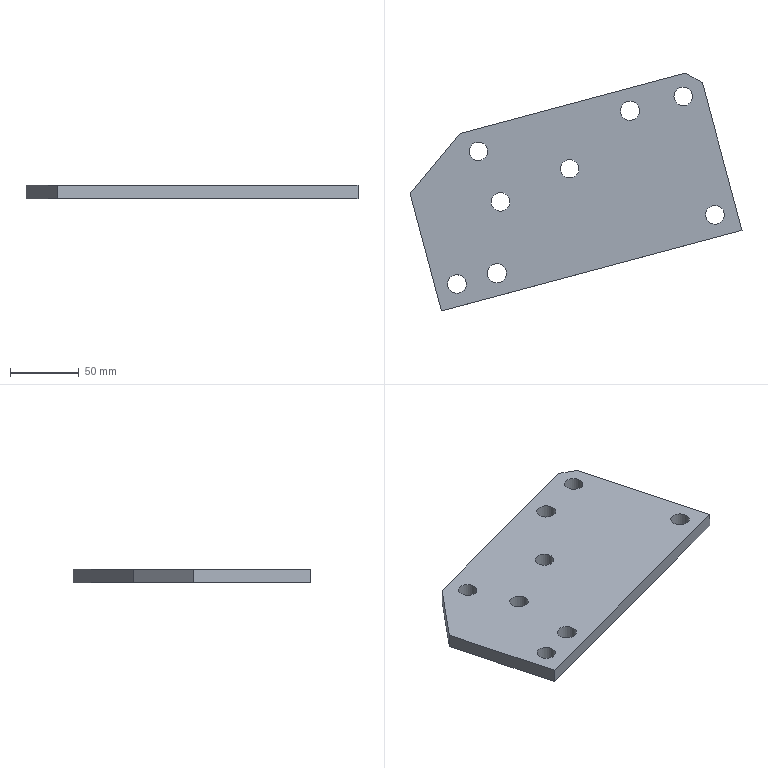Part | NX | features 6 2 | 1 solid | 16 faces | box 241.063 x 172.782 x 10 mm | volume 253614 mm3 | plane 8 | cylinder 8 | commonest cylinder face diameters 13.5 x6 14.001 x2
STEP:
#1=CARTESIAN_POINT('',(606.241,-48.522,101.));
#2=VERTEX_POINT('',#1);
#3=CARTESIAN_POINT('',(599.491,-48.522,101.));
#4=DIRECTION('',(0.,0.,1.));
#5=DIRECTION('',(1.,0.,0.));
#6=AXIS2_PLACEMENT_3D('',#3,#4,#5);
#7=CIRCLE('',#6,6.75);
#8=EDGE_CURVE('',#2,#2,#7,.T.);
#9=ORIENTED_EDGE('',*,*,#8,.F.);
#10=EDGE_LOOP('',(#9));
#11=FACE_BOUND('',#10,.T.);
#12=CARTESIAN_POINT('',(570.07,1.105,101.));
#13=VERTEX_POINT('',#12);
#14=CARTESIAN_POINT('',(533.734,-42.843,101.));
#15=VERTEX_POINT('',#14);
#16=CARTESIAN_POINT('',(534.187,-42.295,101.));
#17=DIRECTION('',(-0.6372,-0.7707,0.));
#18=VECTOR('',#17,1000.);
#19=LINE('',#16,#18);
#20=EDGE_CURVE('',#13,#15,#19,.T.);
#21=ORIENTED_EDGE('',*,*,#20,.T.);
#22=CARTESIAN_POINT('',(556.498,-127.8,101.));
#23=VERTEX_POINT('',#22);
#24=CARTESIAN_POINT('',(542.781,-76.606,101.));
#25=DIRECTION('',(-0.2588,0.9659,0.));
#26=VECTOR('',#25,1000.);
#27=LINE('',#24,#26);
#28=EDGE_CURVE('',#23,#15,#27,.T.);
#29=ORIENTED_EDGE('',*,*,#28,.F.);
#30=CARTESIAN_POINT('',(774.797,-69.307,101.));
#31=VERTEX_POINT('',#30);
#32=CARTESIAN_POINT('',(665.648,-98.554,101.));
#33=DIRECTION('',(-0.9659,-0.2588,0.));
#34=VECTOR('',#33,1000.);
#35=LINE('',#32,#34);
#36=EDGE_CURVE('',#31,#23,#35,.T.);
#37=ORIENTED_EDGE('',*,*,#36,.F.);
#38=CARTESIAN_POINT('',(746.068,37.911,101.));
#39=VERTEX_POINT('',#38);
#40=CARTESIAN_POINT('',(761.08,-18.113,101.));
#41=DIRECTION('',(0.2588,-0.9659,0.));
#42=VECTOR('',#41,1000.);
#43=LINE('',#40,#42);
#44=EDGE_CURVE('',#39,#31,#43,.T.);
#45=ORIENTED_EDGE('',*,*,#44,.F.);
#46=CARTESIAN_POINT('',(733.821,44.982,101.));
#47=VERTEX_POINT('',#46);
#48=CARTESIAN_POINT('',(304.806,292.674,101.));
#49=DIRECTION('',(-0.866,0.5,0.));
#50=VECTOR('',#49,1000.);
#51=LINE('',#48,#50);
#52=EDGE_CURVE('',#39,#47,#51,.T.);
#53=ORIENTED_EDGE('',*,*,#52,.T.);
#54=CARTESIAN_POINT('',(634.331,18.323,101.));
#55=DIRECTION('',(0.9659,0.2588,0.));
#56=VECTOR('',#55,1000.);
#57=LINE('',#54,#56);
#58=EDGE_CURVE('',#13,#47,#57,.T.);
#59=ORIENTED_EDGE('',*,*,#58,.F.);
#60=EDGE_LOOP('',(#21,#29,#37,#45,#53,#59));
#61=FACE_BOUND('',#60,.T.);
#62=CARTESIAN_POINT('',(603.552,-98.628,101.));
#63=VERTEX_POINT('',#62);
#64=CARTESIAN_POINT('',(596.79,-100.44,101.));
#65=DIRECTION('',(0.,0.,-1.));
#66=DIRECTION('',(0.9659,0.2588,0.));
#67=AXIS2_PLACEMENT_3D('',#64,#65,#66);
#68=CIRCLE('',#67,7.);
#69=EDGE_CURVE('',#63,#63,#68,.T.);
#70=ORIENTED_EDGE('',*,*,#69,.T.);
#71=EDGE_LOOP('',(#70));
#72=FACE_BOUND('',#71,.T.);
#73=CARTESIAN_POINT('',(761.721,-56.246,101.));
#74=VERTEX_POINT('',#73);
#75=CARTESIAN_POINT('',(755.201,-57.993,101.));
#76=DIRECTION('',(0.,0.,-1.));
#77=DIRECTION('',(0.9659,0.2588,0.));
#78=AXIS2_PLACEMENT_3D('',#75,#76,#77);
#79=CIRCLE('',#78,6.75);
#80=EDGE_CURVE('',#74,#74,#79,.T.);
#81=ORIENTED_EDGE('',*,*,#80,.T.);
#82=EDGE_LOOP('',(#81));
#83=FACE_BOUND('',#82,.T.);
#84=CARTESIAN_POINT('',(574.332,-106.457,101.));
#85=VERTEX_POINT('',#84);
#86=CARTESIAN_POINT('',(567.812,-108.204,101.));
#87=DIRECTION('',(0.,0.,-1.));
#88=DIRECTION('',(0.9659,0.2588,0.));
#89=AXIS2_PLACEMENT_3D('',#86,#87,#88);
#90=CIRCLE('',#89,6.75);
#91=EDGE_CURVE('',#85,#85,#90,.T.);
#92=ORIENTED_EDGE('',*,*,#91,.T.);
#93=EDGE_LOOP('',(#92));
#94=FACE_BOUND('',#93,.T.);
#95=CARTESIAN_POINT('',(738.687,29.721,101.));
#96=VERTEX_POINT('',#95);
#97=CARTESIAN_POINT('',(732.167,27.974,101.));
#98=DIRECTION('',(0.,0.,-1.));
#99=DIRECTION('',(0.9659,0.2588,0.));
#100=AXIS2_PLACEMENT_3D('',#97,#98,#99);
#101=CIRCLE('',#100,6.75);
#102=EDGE_CURVE('',#96,#96,#101,.T.);
#103=ORIENTED_EDGE('',*,*,#102,.T.);
#104=EDGE_LOOP('',(#103));
#105=FACE_BOUND('',#104,.T.);
#106=CARTESIAN_POINT('',(589.934,-10.137,101.));
#107=VERTEX_POINT('',#106);
#108=CARTESIAN_POINT('',(583.414,-11.884,101.));
#109=DIRECTION('',(0.,0.,-1.));
#110=DIRECTION('',(0.9659,0.2588,0.));
#111=AXIS2_PLACEMENT_3D('',#108,#109,#110);
#112=CIRCLE('',#111,6.75);
#113=EDGE_CURVE('',#107,#107,#112,.T.);
#114=ORIENTED_EDGE('',*,*,#113,.T.);
#115=EDGE_LOOP('',(#114));
#116=FACE_BOUND('',#115,.T.);
#117=CARTESIAN_POINT('',(700.292,19.433,101.));
#118=VERTEX_POINT('',#117);
#119=CARTESIAN_POINT('',(693.53,17.621,101.));
#120=DIRECTION('',(0.,0.,-1.));
#121=DIRECTION('',(0.9659,0.2588,0.));
#122=AXIS2_PLACEMENT_3D('',#119,#120,#121);
#123=CIRCLE('',#122,7.);
#124=EDGE_CURVE('',#118,#118,#123,.T.);
#125=ORIENTED_EDGE('',*,*,#124,.T.);
#126=EDGE_LOOP('',(#125));
#127=FACE_BOUND('',#126,.T.);
#128=CARTESIAN_POINT('',(656.441,-24.522,101.));
#129=VERTEX_POINT('',#128);
#130=CARTESIAN_POINT('',(649.691,-24.522,101.));
#131=DIRECTION('',(0.,0.,1.));
#132=DIRECTION('',(1.,0.,0.));
#133=AXIS2_PLACEMENT_3D('',#130,#131,#132);
#134=CIRCLE('',#133,6.75);
#135=EDGE_CURVE('',#129,#129,#134,.T.);
#136=ORIENTED_EDGE('',*,*,#135,.F.);
#137=EDGE_LOOP('',(#136));
#138=FACE_BOUND('',#137,.T.);
#139=CARTESIAN_POINT('',(189.696,93.298,101.));
#140=DIRECTION('',(0.,0.,1.));
#141=DIRECTION('',(-0.9848,0.1736,0.));
#142=AXIS2_PLACEMENT_3D('',#139,#140,#141);
#143=PLANE('',#142);
#144=ADVANCED_FACE('',(#11,#61,#72,#83,#94,#105,#116,#127,#138),#143,.T.);
#145=CARTESIAN_POINT('',(592.741,-48.522,91.));
#146=VERTEX_POINT('',#145);
#147=CARTESIAN_POINT('',(599.491,-48.522,91.));
#148=DIRECTION('',(0.,0.,1.));
#149=DIRECTION('',(-1.,0.,0.));
#150=AXIS2_PLACEMENT_3D('',#147,#148,#149);
#151=CIRCLE('',#150,6.75);
#152=EDGE_CURVE('',#146,#146,#151,.T.);
#153=ORIENTED_EDGE('',*,*,#152,.T.);
#154=EDGE_LOOP('',(#153));
#155=FACE_BOUND('',#154,.T.);
#156=CARTESIAN_POINT('',(570.07,1.105,91.));
#157=VERTEX_POINT('',#156);
#158=CARTESIAN_POINT('',(533.734,-42.843,91.));
#159=VERTEX_POINT('',#158);
#160=CARTESIAN_POINT('',(579.507,12.519,91.));
#161=DIRECTION('',(-0.6372,-0.7707,0.));
#162=VECTOR('',#161,1000.);
#163=LINE('',#160,#162);
#164=EDGE_CURVE('',#157,#159,#163,.T.);
#165=ORIENTED_EDGE('',*,*,#164,.F.);
#166=CARTESIAN_POINT('',(733.821,44.982,91.));
#167=VERTEX_POINT('',#166);
#168=CARTESIAN_POINT('',(634.331,18.323,91.));
#169=DIRECTION('',(-0.9659,-0.2588,0.));
#170=VECTOR('',#169,1000.);
#171=LINE('',#168,#170);
#172=EDGE_CURVE('',#167,#157,#171,.T.);
#173=ORIENTED_EDGE('',*,*,#172,.F.);
#174=CARTESIAN_POINT('',(746.068,37.911,91.));
#175=VERTEX_POINT('',#174);
#176=CARTESIAN_POINT('',(712.388,57.356,91.));
#177=DIRECTION('',(0.866,-0.5,0.));
#178=VECTOR('',#177,1000.);
#179=LINE('',#176,#178);
#180=EDGE_CURVE('',#167,#175,#179,.T.);
#181=ORIENTED_EDGE('',*,*,#180,.T.);
#182=CARTESIAN_POINT('',(774.797,-69.307,91.));
#183=VERTEX_POINT('',#182);
#184=CARTESIAN_POINT('',(761.08,-18.113,91.));
#185=DIRECTION('',(-0.2588,0.9659,0.));
#186=VECTOR('',#185,1000.);
#187=LINE('',#184,#186);
#188=EDGE_CURVE('',#183,#175,#187,.T.);
#189=ORIENTED_EDGE('',*,*,#188,.F.);
#190=CARTESIAN_POINT('',(556.498,-127.8,91.));
#191=VERTEX_POINT('',#190);
#192=CARTESIAN_POINT('',(665.648,-98.554,91.));
#193=DIRECTION('',(0.9659,0.2588,0.));
#194=VECTOR('',#193,1000.);
#195=LINE('',#192,#194);
#196=EDGE_CURVE('',#191,#183,#195,.T.);
#197=ORIENTED_EDGE('',*,*,#196,.F.);
#198=CARTESIAN_POINT('',(542.781,-76.606,91.));
#199=DIRECTION('',(0.2588,-0.9659,0.));
#200=VECTOR('',#199,1000.);
#201=LINE('',#198,#200);
#202=EDGE_CURVE('',#159,#191,#201,.T.);
#203=ORIENTED_EDGE('',*,*,#202,.F.);
#204=EDGE_LOOP('',(#165,#173,#181,#189,#197,#203));
#205=FACE_BOUND('',#204,.T.);
#206=CARTESIAN_POINT('',(603.552,-98.628,91.));
#207=VERTEX_POINT('',#206);
#208=CARTESIAN_POINT('',(596.79,-100.44,91.));
#209=DIRECTION('',(0.,0.,1.));
#210=DIRECTION('',(0.9659,0.2588,0.));
#211=AXIS2_PLACEMENT_3D('',#208,#209,#210);
#212=CIRCLE('',#211,7.);
#213=EDGE_CURVE('',#207,#207,#212,.T.);
#214=ORIENTED_EDGE('',*,*,#213,.T.);
#215=EDGE_LOOP('',(#214));
#216=FACE_BOUND('',#215,.T.);
#217=CARTESIAN_POINT('',(761.721,-56.246,91.));
#218=VERTEX_POINT('',#217);
#219=CARTESIAN_POINT('',(755.201,-57.993,91.));
#220=DIRECTION('',(0.,0.,1.));
#221=DIRECTION('',(0.9659,0.2588,0.));
#222=AXIS2_PLACEMENT_3D('',#219,#220,#221);
#223=CIRCLE('',#222,6.75);
#224=EDGE_CURVE('',#218,#218,#223,.T.);
#225=ORIENTED_EDGE('',*,*,#224,.T.);
#226=EDGE_LOOP('',(#225));
#227=FACE_BOUND('',#226,.T.);
#228=CARTESIAN_POINT('',(574.332,-106.457,91.));
#229=VERTEX_POINT('',#228);
#230=CARTESIAN_POINT('',(567.812,-108.204,91.));
#231=DIRECTION('',(0.,0.,1.));
#232=DIRECTION('',(0.9659,0.2588,0.));
#233=AXIS2_PLACEMENT_3D('',#230,#231,#232);
#234=CIRCLE('',#233,6.75);
#235=EDGE_CURVE('',#229,#229,#234,.T.);
#236=ORIENTED_EDGE('',*,*,#235,.T.);
#237=EDGE_LOOP('',(#236));
#238=FACE_BOUND('',#237,.T.);
#239=CARTESIAN_POINT('',(738.687,29.721,91.));
#240=VERTEX_POINT('',#239);
#241=CARTESIAN_POINT('',(732.167,27.974,91.));
#242=DIRECTION('',(0.,0.,1.));
#243=DIRECTION('',(0.9659,0.2588,0.));
#244=AXIS2_PLACEMENT_3D('',#241,#242,#243);
#245=CIRCLE('',#244,6.75);
#246=EDGE_CURVE('',#240,#240,#245,.T.);
#247=ORIENTED_EDGE('',*,*,#246,.T.);
#248=EDGE_LOOP('',(#247));
#249=FACE_BOUND('',#248,.T.);
#250=CARTESIAN_POINT('',(589.934,-10.137,91.));
#251=VERTEX_POINT('',#250);
#252=CARTESIAN_POINT('',(583.414,-11.884,91.));
#253=DIRECTION('',(0.,0.,1.));
#254=DIRECTION('',(0.9659,0.2588,0.));
#255=AXIS2_PLACEMENT_3D('',#252,#253,#254);
#256=CIRCLE('',#255,6.75);
#257=EDGE_CURVE('',#251,#251,#256,.T.);
#258=ORIENTED_EDGE('',*,*,#257,.T.);
#259=EDGE_LOOP('',(#258));
#260=FACE_BOUND('',#259,.T.);
#261=CARTESIAN_POINT('',(700.292,19.433,91.));
#262=VERTEX_POINT('',#261);
#263=CARTESIAN_POINT('',(693.53,17.621,91.));
#264=DIRECTION('',(0.,0.,1.));
#265=DIRECTION('',(0.9659,0.2588,0.));
#266=AXIS2_PLACEMENT_3D('',#263,#264,#265);
#267=CIRCLE('',#266,7.);
#268=EDGE_CURVE('',#262,#262,#267,.T.);
#269=ORIENTED_EDGE('',*,*,#268,.T.);
#270=EDGE_LOOP('',(#269));
#271=FACE_BOUND('',#270,.T.);
#272=CARTESIAN_POINT('',(642.941,-24.522,91.));
#273=VERTEX_POINT('',#272);
#274=CARTESIAN_POINT('',(649.691,-24.522,91.));
#275=DIRECTION('',(0.,0.,1.));
#276=DIRECTION('',(-1.,0.,0.));
#277=AXIS2_PLACEMENT_3D('',#274,#275,#276);
#278=CIRCLE('',#277,6.75);
#279=EDGE_CURVE('',#273,#273,#278,.T.);
#280=ORIENTED_EDGE('',*,*,#279,.T.);
#281=EDGE_LOOP('',(#280));
#282=FACE_BOUND('',#281,.T.);
#283=CARTESIAN_POINT('',(651.93,-47.36,91.));
#284=DIRECTION('',(0.,0.,-1.));
#285=DIRECTION('',(0.9659,0.2588,0.));
#286=AXIS2_PLACEMENT_3D('',#283,#284,#285);
#287=PLANE('',#286);
#288=ADVANCED_FACE('',(#155,#205,#216,#227,#238,#249,#260,#271,#282),#287,.T.);
#289=CARTESIAN_POINT('',(774.797,-69.307,91.));
#290=DIRECTION('',(0.,0.,1.));
#291=VECTOR('',#290,1000.);
#292=LINE('',#289,#291);
#293=EDGE_CURVE('',#183,#31,#292,.T.);
#294=ORIENTED_EDGE('',*,*,#293,.T.);
#295=ORIENTED_EDGE('',*,*,#36,.T.);
#296=CARTESIAN_POINT('',(556.498,-127.8,91.));
#297=DIRECTION('',(0.,0.,1.));
#298=VECTOR('',#297,1000.);
#299=LINE('',#296,#298);
#300=EDGE_CURVE('',#191,#23,#299,.T.);
#301=ORIENTED_EDGE('',*,*,#300,.F.);
#302=ORIENTED_EDGE('',*,*,#196,.T.);
#303=EDGE_LOOP('',(#294,#295,#301,#302));
#304=FACE_BOUND('',#303,.T.);
#305=CARTESIAN_POINT('',(665.648,-98.554,91.));
#306=DIRECTION('',(0.2588,-0.9659,0.));
#307=DIRECTION('',(0.,0.,1.));
#308=AXIS2_PLACEMENT_3D('',#305,#306,#307);
#309=PLANE('',#308);
#310=ADVANCED_FACE('',(#304),#309,.T.);
#311=CARTESIAN_POINT('',(533.734,-42.843,91.));
#312=DIRECTION('',(0.,0.,1.));
#313=VECTOR('',#312,1000.);
#314=LINE('',#311,#313);
#315=EDGE_CURVE('',#159,#15,#314,.T.);
#316=ORIENTED_EDGE('',*,*,#315,.F.);
#317=ORIENTED_EDGE('',*,*,#202,.T.);
#318=ORIENTED_EDGE('',*,*,#300,.T.);
#319=ORIENTED_EDGE('',*,*,#28,.T.);
#320=EDGE_LOOP('',(#316,#317,#318,#319));
#321=FACE_BOUND('',#320,.T.);
#322=CARTESIAN_POINT('',(542.781,-76.606,91.));
#323=DIRECTION('',(-0.9659,-0.2588,0.));
#324=DIRECTION('',(0.,0.,-1.));
#325=AXIS2_PLACEMENT_3D('',#322,#323,#324);
#326=PLANE('',#325);
#327=ADVANCED_FACE('',(#321),#326,.T.);
#328=CARTESIAN_POINT('',(570.07,1.105,91.));
#329=DIRECTION('',(0.,0.,-1.));
#330=VECTOR('',#329,1000.);
#331=LINE('',#328,#330);
#332=EDGE_CURVE('',#13,#157,#331,.T.);
#333=ORIENTED_EDGE('',*,*,#332,.F.);
#334=ORIENTED_EDGE('',*,*,#58,.T.);
#335=CARTESIAN_POINT('',(733.821,44.982,91.));
#336=DIRECTION('',(0.,0.,-1.));
#337=VECTOR('',#336,1000.);
#338=LINE('',#335,#337);
#339=EDGE_CURVE('',#47,#167,#338,.T.);
#340=ORIENTED_EDGE('',*,*,#339,.T.);
#341=ORIENTED_EDGE('',*,*,#172,.T.);
#342=EDGE_LOOP('',(#333,#334,#340,#341));
#343=FACE_BOUND('',#342,.T.);
#344=CARTESIAN_POINT('',(634.331,18.323,91.));
#345=DIRECTION('',(-0.2588,0.9659,0.));
#346=DIRECTION('',(0.,0.,-1.));
#347=AXIS2_PLACEMENT_3D('',#344,#345,#346);
#348=PLANE('',#347);
#349=ADVANCED_FACE('',(#343),#348,.T.);
#350=ORIENTED_EDGE('',*,*,#188,.T.);
#351=CARTESIAN_POINT('',(746.068,37.911,91.));
#352=DIRECTION('',(0.,0.,1.));
#353=VECTOR('',#352,1000.);
#354=LINE('',#351,#353);
#355=EDGE_CURVE('',#175,#39,#354,.T.);
#356=ORIENTED_EDGE('',*,*,#355,.T.);
#357=ORIENTED_EDGE('',*,*,#44,.T.);
#358=ORIENTED_EDGE('',*,*,#293,.F.);
#359=EDGE_LOOP('',(#350,#356,#357,#358));
#360=FACE_BOUND('',#359,.T.);
#361=CARTESIAN_POINT('',(761.08,-18.113,91.));
#362=DIRECTION('',(0.9659,0.2588,0.));
#363=DIRECTION('',(0.,0.,1.));
#364=AXIS2_PLACEMENT_3D('',#361,#362,#363);
#365=PLANE('',#364);
#366=ADVANCED_FACE('',(#360),#365,.T.);
#367=ORIENTED_EDGE('',*,*,#91,.F.);
#368=EDGE_LOOP('',(#367));
#369=FACE_BOUND('',#368,.T.);
#370=ORIENTED_EDGE('',*,*,#235,.F.);
#371=EDGE_LOOP('',(#370));
#372=FACE_BOUND('',#371,.T.);
#373=CARTESIAN_POINT('',(567.812,-108.204,91.));
#374=DIRECTION('',(0.,0.,1.));
#375=DIRECTION('',(-0.9659,-0.2588,0.));
#376=AXIS2_PLACEMENT_3D('',#373,#374,#375);
#377=CYLINDRICAL_SURFACE('',#376,6.75);
#378=ADVANCED_FACE('',(#369,#372),#377,.F.);
#379=ORIENTED_EDGE('',*,*,#102,.F.);
#380=EDGE_LOOP('',(#379));
#381=FACE_BOUND('',#380,.T.);
#382=ORIENTED_EDGE('',*,*,#246,.F.);
#383=EDGE_LOOP('',(#382));
#384=FACE_BOUND('',#383,.T.);
#385=CARTESIAN_POINT('',(732.167,27.974,91.));
#386=DIRECTION('',(0.,0.,1.));
#387=DIRECTION('',(-0.9659,-0.2588,0.));
#388=AXIS2_PLACEMENT_3D('',#385,#386,#387);
#389=CYLINDRICAL_SURFACE('',#388,6.75);
#390=ADVANCED_FACE('',(#381,#384),#389,.F.);
#391=ORIENTED_EDGE('',*,*,#80,.F.);
#392=EDGE_LOOP('',(#391));
#393=FACE_BOUND('',#392,.T.);
#394=ORIENTED_EDGE('',*,*,#224,.F.);
#395=EDGE_LOOP('',(#394));
#396=FACE_BOUND('',#395,.T.);
#397=CARTESIAN_POINT('',(755.201,-57.993,91.));
#398=DIRECTION('',(0.,0.,1.));
#399=DIRECTION('',(-0.9659,-0.2588,0.));
#400=AXIS2_PLACEMENT_3D('',#397,#398,#399);
#401=CYLINDRICAL_SURFACE('',#400,6.75);
#402=ADVANCED_FACE('',(#393,#396),#401,.F.);
#403=ORIENTED_EDGE('',*,*,#113,.F.);
#404=EDGE_LOOP('',(#403));
#405=FACE_BOUND('',#404,.T.);
#406=ORIENTED_EDGE('',*,*,#257,.F.);
#407=EDGE_LOOP('',(#406));
#408=FACE_BOUND('',#407,.T.);
#409=CARTESIAN_POINT('',(583.414,-11.884,91.));
#410=DIRECTION('',(0.,0.,1.));
#411=DIRECTION('',(-0.9659,-0.2588,0.));
#412=AXIS2_PLACEMENT_3D('',#409,#410,#411);
#413=CYLINDRICAL_SURFACE('',#412,6.75);
#414=ADVANCED_FACE('',(#405,#408),#413,.F.);
#415=ORIENTED_EDGE('',*,*,#69,.F.);
#416=EDGE_LOOP('',(#415));
#417=FACE_BOUND('',#416,.T.);
#418=ORIENTED_EDGE('',*,*,#213,.F.);
#419=EDGE_LOOP('',(#418));
#420=FACE_BOUND('',#419,.T.);
#421=CARTESIAN_POINT('',(596.79,-100.44,91.));
#422=DIRECTION('',(0.,0.,1.));
#423=DIRECTION('',(-0.9659,-0.2588,0.));
#424=AXIS2_PLACEMENT_3D('',#421,#422,#423);
#425=CYLINDRICAL_SURFACE('',#424,7.);
#426=ADVANCED_FACE('',(#417,#420),#425,.F.);
#427=ORIENTED_EDGE('',*,*,#124,.F.);
#428=EDGE_LOOP('',(#427));
#429=FACE_BOUND('',#428,.T.);
#430=ORIENTED_EDGE('',*,*,#268,.F.);
#431=EDGE_LOOP('',(#430));
#432=FACE_BOUND('',#431,.T.);
#433=CARTESIAN_POINT('',(693.53,17.621,91.));
#434=DIRECTION('',(0.,0.,1.));
#435=DIRECTION('',(-0.9659,-0.2588,0.));
#436=AXIS2_PLACEMENT_3D('',#433,#434,#435);
#437=CYLINDRICAL_SURFACE('',#436,7.);
#438=ADVANCED_FACE('',(#429,#432),#437,.F.);
#439=ORIENTED_EDGE('',*,*,#180,.F.);
#440=ORIENTED_EDGE('',*,*,#339,.F.);
#441=ORIENTED_EDGE('',*,*,#52,.F.);
#442=ORIENTED_EDGE('',*,*,#355,.F.);
#443=EDGE_LOOP('',(#439,#440,#441,#442));
#444=FACE_BOUND('',#443,.T.);
#445=CARTESIAN_POINT('',(746.068,37.911,91.));
#446=DIRECTION('',(-0.5,-0.866,0.));
#447=DIRECTION('',(0.,0.,-1.));
#448=AXIS2_PLACEMENT_3D('',#445,#446,#447);
#449=PLANE('',#448);
#450=ADVANCED_FACE('',(#444),#449,.F.);
#451=ORIENTED_EDGE('',*,*,#20,.F.);
#452=ORIENTED_EDGE('',*,*,#332,.T.);
#453=ORIENTED_EDGE('',*,*,#164,.T.);
#454=ORIENTED_EDGE('',*,*,#315,.T.);
#455=EDGE_LOOP('',(#451,#452,#453,#454));
#456=FACE_BOUND('',#455,.T.);
#457=CARTESIAN_POINT('',(534.187,-42.295,-36.));
#458=DIRECTION('',(0.7707,-0.6372,0.));
#459=DIRECTION('',(-0.6372,-0.7707,0.));
#460=AXIS2_PLACEMENT_3D('',#457,#458,#459);
#461=PLANE('',#460);
#462=ADVANCED_FACE('',(#456),#461,.F.);
#463=ORIENTED_EDGE('',*,*,#8,.T.);
#464=EDGE_LOOP('',(#463));
#465=FACE_BOUND('',#464,.T.);
#466=ORIENTED_EDGE('',*,*,#152,.F.);
#467=EDGE_LOOP('',(#466));
#468=FACE_BOUND('',#467,.T.);
#469=CARTESIAN_POINT('',(599.491,-48.522,-196.));
#470=DIRECTION('',(0.,0.,1.));
#471=DIRECTION('',(-1.,0.,0.));
#472=AXIS2_PLACEMENT_3D('',#469,#470,#471);
#473=CYLINDRICAL_SURFACE('',#472,6.75);
#474=ADVANCED_FACE('',(#465,#468),#473,.F.);
#475=ORIENTED_EDGE('',*,*,#135,.T.);
#476=EDGE_LOOP('',(#475));
#477=FACE_BOUND('',#476,.T.);
#478=ORIENTED_EDGE('',*,*,#279,.F.);
#479=EDGE_LOOP('',(#478));
#480=FACE_BOUND('',#479,.T.);
#481=CARTESIAN_POINT('',(649.691,-24.522,-196.));
#482=DIRECTION('',(0.,0.,1.));
#483=DIRECTION('',(-1.,0.,0.));
#484=AXIS2_PLACEMENT_3D('',#481,#482,#483);
#485=CYLINDRICAL_SURFACE('',#484,6.75);
#486=ADVANCED_FACE('',(#477,#480),#485,.F.);
#487=CLOSED_SHELL('',(#144,#288,#310,#327,#349,#366,#378,#390,#402,#414,#426,#438,#450,#462,#474,#486));
#488=MANIFOLD_SOLID_BREP('',#487);
#489=(LENGTH_UNIT()NAMED_UNIT(*)SI_UNIT(.MILLI.,.METRE.));
#490=UNCERTAINTY_MEASURE_WITH_UNIT(LENGTH_MEASURE(0.00001),#489,'','');
#491=(NAMED_UNIT(*)PLANE_ANGLE_UNIT()SI_UNIT($,.RADIAN.));
#492=(NAMED_UNIT(*)SI_UNIT($,.STERADIAN.)SOLID_ANGLE_UNIT());
#493=(GEOMETRIC_REPRESENTATION_CONTEXT(3)GLOBAL_UNCERTAINTY_ASSIGNED_CONTEXT((#490))GLOBAL_UNIT_ASSIGNED_CONTEXT((#489,#491,#492))REPRESENTATION_CONTEXT('',''));
#494=ADVANCED_BREP_SHAPE_REPRESENTATION('',(#488),#493);